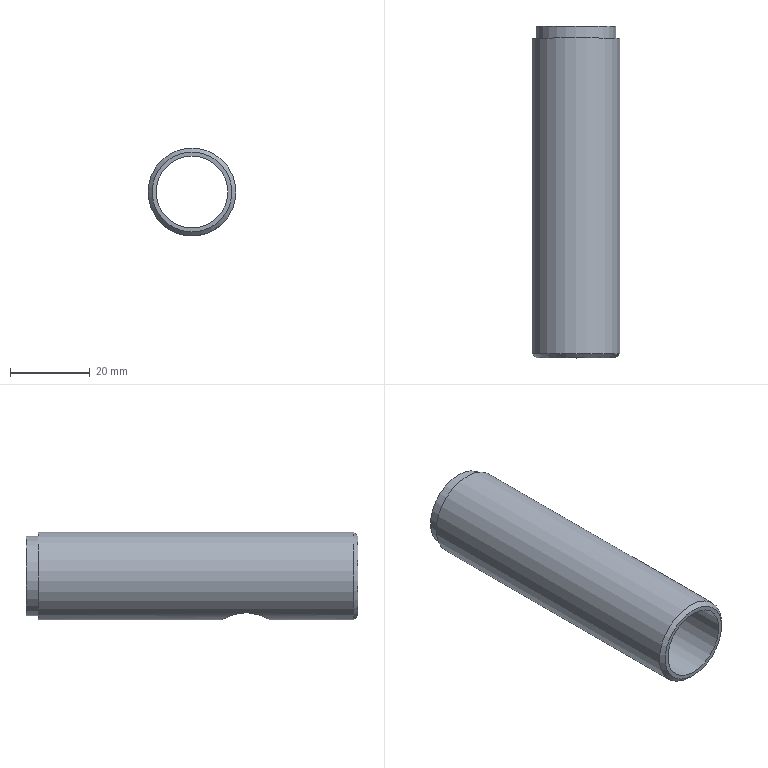Part | STEP file | JBJ-P-1012-04 | 1 solid | 8 faces | box 22 x 83 x 22 mm | volume 9931 mm3 | cylinder 4 | plane 2 | cone 2 | commonest cylinder face diameters 12 x1 18 x1 20 x1 22 x1
STEP:
#1=CARTESIAN_POINT('',(0.,0.,-10.));
#2=VERTEX_POINT('',#1);
#3=CARTESIAN_POINT('',(0.,0.,0.));
#4=DIRECTION('',(0.,-1.,0.));
#5=DIRECTION('',(0.,0.,-1.));
#6=AXIS2_PLACEMENT_3D('',#3,#4,#5);
#7=CIRCLE('',#6,10.);
#8=EDGE_CURVE('',#2,#2,#7,.T.);
#9=ORIENTED_EDGE('',*,*,#8,.T.);
#10=EDGE_LOOP('',(#9));
#11=FACE_OUTER_BOUND('',#10,.T.);
#12=CARTESIAN_POINT('',(0.,0.,-9.));
#13=VERTEX_POINT('',#12);
#14=CARTESIAN_POINT('',(0.,0.,0.));
#15=DIRECTION('',(0.,-1.,0.));
#16=DIRECTION('',(0.,0.,-1.));
#17=AXIS2_PLACEMENT_3D('',#14,#15,#16);
#18=CIRCLE('',#17,9.);
#19=EDGE_CURVE('',#13,#13,#18,.T.);
#20=ORIENTED_EDGE('',*,*,#19,.F.);
#21=EDGE_LOOP('',(#20));
#22=FACE_BOUND('',#21,.T.);
#23=CARTESIAN_POINT('',(11.,0.,0.));
#24=DIRECTION('',(0.,-1.,0.));
#25=DIRECTION('',(0.,0.,-1.));
#26=AXIS2_PLACEMENT_3D('',#23,#24,#25);
#27=PLANE('',#26);
#28=ADVANCED_FACE('',(#11,#22),#27,.T.);
#29=CARTESIAN_POINT('',(0.,34.,-9.));
#30=VERTEX_POINT('',#29);
#31=CARTESIAN_POINT('',(0.,34.,-9.));
#32=CARTESIAN_POINT('',(-0.4103,34.,-9.));
#33=CARTESIAN_POINT('',(-0.8115,33.958,-8.972));
#34=CARTESIAN_POINT('',(-1.597,33.797,-8.866));
#35=CARTESIAN_POINT('',(-1.985,33.676,-8.786));
#36=CARTESIAN_POINT('',(-2.708,33.368,-8.591));
#37=CARTESIAN_POINT('',(-3.05,33.182,-8.475));
#38=CARTESIAN_POINT('',(-3.692,32.746,-8.215));
#39=CARTESIAN_POINT('',(-3.984,32.502,-8.076));
#40=CARTESIAN_POINT('',(-4.519,31.965,-7.789));
#41=CARTESIAN_POINT('',(-4.763,31.668,-7.64));
#42=CARTESIAN_POINT('',(-5.188,31.039,-7.359));
#43=CARTESIAN_POINT('',(-5.37,30.705,-7.225));
#44=CARTESIAN_POINT('',(-5.673,29.992,-6.99));
#45=CARTESIAN_POINT('',(-5.794,29.609,-6.888));
#46=CARTESIAN_POINT('',(-5.916,29.023,-6.783));
#47=CARTESIAN_POINT('',(-5.947,28.825,-6.756));
#48=CARTESIAN_POINT('',(-5.989,28.421,-6.718));
#49=CARTESIAN_POINT('',(-6.,28.215,-6.709));
#50=CARTESIAN_POINT('',(-6.001,27.605,-6.708));
#51=CARTESIAN_POINT('',(-5.961,27.204,-6.744));
#52=CARTESIAN_POINT('',(-5.8,26.413,-6.882));
#53=CARTESIAN_POINT('',(-5.682,26.035,-6.982));
#54=CARTESIAN_POINT('',(-5.38,25.316,-7.217));
#55=CARTESIAN_POINT('',(-5.195,24.974,-7.354));
#56=CARTESIAN_POINT('',(-4.771,24.342,-7.636));
#57=CARTESIAN_POINT('',(-4.529,24.046,-7.783));
#58=CARTESIAN_POINT('',(-3.992,23.504,-8.072));
#59=CARTESIAN_POINT('',(-3.7,23.261,-8.211));
#60=CARTESIAN_POINT('',(-3.226,22.937,-8.404));
#61=CARTESIAN_POINT('',(-3.061,22.836,-8.465));
#62=CARTESIAN_POINT('',(-2.719,22.648,-8.581));
#63=CARTESIAN_POINT('',(-2.54,22.561,-8.636));
#64=CARTESIAN_POINT('',(-1.996,22.328,-8.784));
#65=CARTESIAN_POINT('',(-1.617,22.208,-8.863));
#66=CARTESIAN_POINT('',(-1.023,22.084,-8.944));
#67=CARTESIAN_POINT('',(-0.8202,22.053,-8.965));
#68=CARTESIAN_POINT('',(-0.4168,22.011,-8.993));
#69=CARTESIAN_POINT('',(-0.01304,21.99,-9.007));
#70=CARTESIAN_POINT('',(0.3916,22.009,-8.994));
#71=CARTESIAN_POINT('',(0.7967,22.05,-8.967));
#72=CARTESIAN_POINT('',(0.9997,22.08,-8.947));
#73=CARTESIAN_POINT('',(1.593,22.201,-8.867));
#74=CARTESIAN_POINT('',(1.973,22.32,-8.789));
#75=CARTESIAN_POINT('',(2.705,22.63,-8.592));
#76=CARTESIAN_POINT('',(3.048,22.818,-8.475));
#77=CARTESIAN_POINT('',(3.686,23.25,-8.218));
#78=CARTESIAN_POINT('',(3.985,23.498,-8.076));
#79=CARTESIAN_POINT('',(4.521,24.037,-7.788));
#80=CARTESIAN_POINT('',(4.761,24.329,-7.642));
#81=CARTESIAN_POINT('',(5.082,24.804,-7.429));
#82=CARTESIAN_POINT('',(5.182,24.969,-7.359));
#83=CARTESIAN_POINT('',(5.366,25.308,-7.227));
#84=CARTESIAN_POINT('',(5.449,25.482,-7.163));
#85=CARTESIAN_POINT('',(5.601,25.839,-7.046));
#86=CARTESIAN_POINT('',(5.668,26.022,-6.991));
#87=CARTESIAN_POINT('',(5.786,26.399,-6.894));
#88=CARTESIAN_POINT('',(5.837,26.595,-6.851));
#89=CARTESIAN_POINT('',(5.958,27.186,-6.746));
#90=CARTESIAN_POINT('',(6.,27.588,-6.708));
#91=CARTESIAN_POINT('',(6.,28.203,-6.708));
#92=CARTESIAN_POINT('',(5.99,28.408,-6.718));
#93=CARTESIAN_POINT('',(5.948,28.81,-6.754));
#94=CARTESIAN_POINT('',(5.918,29.009,-6.781));
#95=CARTESIAN_POINT('',(5.837,29.402,-6.85));
#96=CARTESIAN_POINT('',(5.787,29.597,-6.893));
#97=CARTESIAN_POINT('',(5.669,29.976,-6.991));
#98=CARTESIAN_POINT('',(5.601,30.16,-7.045));
#99=CARTESIAN_POINT('',(5.375,30.695,-7.222));
#100=CARTESIAN_POINT('',(5.192,31.032,-7.356));
#101=CARTESIAN_POINT('',(4.762,31.67,-7.641));
#102=CARTESIAN_POINT('',(4.522,31.962,-7.788));
#103=CARTESIAN_POINT('',(3.986,32.5,-8.075));
#104=CARTESIAN_POINT('',(3.688,32.748,-8.217));
#105=CARTESIAN_POINT('',(3.051,33.181,-8.474));
#106=CARTESIAN_POINT('',(2.713,33.366,-8.59));
#107=CARTESIAN_POINT('',(1.991,33.674,-8.785));
#108=CARTESIAN_POINT('',(1.602,33.796,-8.865));
#109=CARTESIAN_POINT('',(0.814,33.958,-8.972));
#110=CARTESIAN_POINT('',(0.4103,34.,-9.));
#111=CARTESIAN_POINT('',(0.,34.,-9.));
#112=B_SPLINE_CURVE_WITH_KNOTS('',3,(#31,#32,#33,#34,#35,#36,#37,#38,#39,#40,#41,#42,#43,#44,#45,#46,#47,#48,#49,#50,#51,#52,#53,#54,#55,#56,#57,#58,#59,#60,#61,#62,#63,#64,#65,#66,#67,#68,#69,#70,#71,#72,#73,#74,#75,#76,#77,#78,#79,#80,#81,#82,#83,#84,#85,#86,#87,#88,#89,#90,#91,#92,#93,#94,#95,#96,#97,#98,#99,#100,#101,#102,#103,#104,#105,#106,#107,#108,#109,#110,#111),.UNSPECIFIED.,.T.,.F.,(4,2,2,2,2,2,2,2,2,2,2,2,2,2,2,2,2,2,2,1,2,2,2,2,2,2,2,2,2,2,2,2,2,2,2,2,2,2,2,2,4),(0.,0.001211,0.002422,0.003634,0.004845,0.006056,0.007267,0.008478,0.009084,0.00969,0.0109,0.01211,0.01332,0.01453,0.01575,0.01635,0.01696,0.01817,0.01877,0.01938,0.01998,0.02059,0.0218,0.02301,0.02422,0.02543,0.02604,0.02665,0.02725,0.02786,0.02907,0.02967,0.03028,0.03089,0.03149,0.0327,0.03391,0.03512,0.03634,0.03755,0.03876),.UNSPECIFIED.);
#113=EDGE_CURVE('',#30,#30,#112,.T.);
#114=ORIENTED_EDGE('',*,*,#113,.F.);
#115=EDGE_LOOP('',(#114));
#116=FACE_BOUND('',#115,.T.);
#117=CARTESIAN_POINT('',(0.,82.,9.));
#118=VERTEX_POINT('',#117);
#119=CARTESIAN_POINT('',(0.,82.,0.));
#120=DIRECTION('',(0.,1.,0.));
#121=DIRECTION('',(0.,0.,1.));
#122=AXIS2_PLACEMENT_3D('',#119,#120,#121);
#123=CIRCLE('',#122,9.);
#124=EDGE_CURVE('',#118,#118,#123,.T.);
#125=ORIENTED_EDGE('',*,*,#124,.T.);
#126=EDGE_LOOP('',(#125));
#127=FACE_OUTER_BOUND('',#126,.T.);
#128=ORIENTED_EDGE('',*,*,#19,.T.);
#129=EDGE_LOOP('',(#128));
#130=FACE_OUTER_BOUND('',#129,.T.);
#131=CARTESIAN_POINT('',(0.,0.,0.));
#132=DIRECTION('',(0.,-1.,0.));
#133=DIRECTION('',(0.,0.,-1.));
#134=AXIS2_PLACEMENT_3D('',#131,#132,#133);
#135=CYLINDRICAL_SURFACE('',#134,9.);
#136=ADVANCED_FACE('',(#116,#127,#130),#135,.F.);
#137=CARTESIAN_POINT('',(0.,83.,-10.));
#138=VERTEX_POINT('',#137);
#139=CARTESIAN_POINT('',(0.,83.,0.));
#140=DIRECTION('',(0.,-1.,0.));
#141=DIRECTION('',(0.,0.,-1.));
#142=AXIS2_PLACEMENT_3D('',#139,#140,#141);
#143=CIRCLE('',#142,10.);
#144=EDGE_CURVE('',#138,#138,#143,.T.);
#145=ORIENTED_EDGE('',*,*,#144,.T.);
#146=EDGE_LOOP('',(#145));
#147=FACE_OUTER_BOUND('',#146,.T.);
#148=CARTESIAN_POINT('',(0.,80.,-10.));
#149=VERTEX_POINT('',#148);
#150=CARTESIAN_POINT('',(0.,80.,0.));
#151=DIRECTION('',(0.,-1.,0.));
#152=DIRECTION('',(0.,0.,-1.));
#153=AXIS2_PLACEMENT_3D('',#150,#151,#152);
#154=CIRCLE('',#153,10.);
#155=EDGE_CURVE('',#149,#149,#154,.T.);
#156=ORIENTED_EDGE('',*,*,#155,.F.);
#157=EDGE_LOOP('',(#156));
#158=FACE_OUTER_BOUND('',#157,.T.);
#159=CARTESIAN_POINT('',(0.,0.,0.));
#160=DIRECTION('',(0.,-1.,0.));
#161=DIRECTION('',(0.,0.,-1.));
#162=AXIS2_PLACEMENT_3D('',#159,#160,#161);
#163=CYLINDRICAL_SURFACE('',#162,10.);
#164=ADVANCED_FACE('',(#147,#158),#163,.T.);
#165=ORIENTED_EDGE('',*,*,#155,.T.);
#166=EDGE_LOOP('',(#165));
#167=FACE_BOUND('',#166,.T.);
#168=CARTESIAN_POINT('',(0.,80.,-11.));
#169=VERTEX_POINT('',#168);
#170=CARTESIAN_POINT('',(0.,80.,0.));
#171=DIRECTION('',(0.,-1.,0.));
#172=DIRECTION('',(0.,0.,-1.));
#173=AXIS2_PLACEMENT_3D('',#170,#171,#172);
#174=CIRCLE('',#173,11.);
#175=EDGE_CURVE('',#169,#169,#174,.T.);
#176=ORIENTED_EDGE('',*,*,#175,.F.);
#177=EDGE_LOOP('',(#176));
#178=FACE_OUTER_BOUND('',#177,.T.);
#179=CARTESIAN_POINT('',(10.,80.,0.));
#180=DIRECTION('',(0.,1.,0.));
#181=DIRECTION('',(0.,0.,1.));
#182=AXIS2_PLACEMENT_3D('',#179,#180,#181);
#183=PLANE('',#182);
#184=ADVANCED_FACE('',(#167,#178),#183,.T.);
#185=CARTESIAN_POINT('',(0.,34.,-11.));
#186=VERTEX_POINT('',#185);
#187=CARTESIAN_POINT('',(0.,34.,-11.));
#188=CARTESIAN_POINT('',(0.4049,34.,-11.));
#189=CARTESIAN_POINT('',(0.8015,33.959,-10.978));
#190=CARTESIAN_POINT('',(1.58,33.802,-10.893));
#191=CARTESIAN_POINT('',(1.965,33.683,-10.829));
#192=CARTESIAN_POINT('',(2.688,33.378,-10.673));
#193=CARTESIAN_POINT('',(3.03,33.193,-10.58));
#194=CARTESIAN_POINT('',(3.676,32.758,-10.373));
#195=CARTESIAN_POINT('',(3.974,32.511,-10.261));
#196=CARTESIAN_POINT('',(4.38,32.105,-10.091));
#197=CARTESIAN_POINT('',(4.509,31.963,-10.034));
#198=CARTESIAN_POINT('',(4.754,31.665,-9.921));
#199=CARTESIAN_POINT('',(4.87,31.509,-9.864));
#200=CARTESIAN_POINT('',(5.194,31.029,-9.7));
#201=CARTESIAN_POINT('',(5.377,30.69,-9.598));
#202=CARTESIAN_POINT('',(5.604,30.153,-9.466));
#203=CARTESIAN_POINT('',(5.671,29.969,-9.426));
#204=CARTESIAN_POINT('',(5.789,29.59,-9.354));
#205=CARTESIAN_POINT('',(5.839,29.396,-9.323));
#206=CARTESIAN_POINT('',(5.958,28.814,-9.247));
#207=CARTESIAN_POINT('',(5.999,28.42,-9.22));
#208=CARTESIAN_POINT('',(6.001,27.819,-9.219));
#209=CARTESIAN_POINT('',(5.991,27.615,-9.225));
#210=CARTESIAN_POINT('',(5.952,27.216,-9.251));
#211=CARTESIAN_POINT('',(5.922,27.018,-9.27));
#212=CARTESIAN_POINT('',(5.845,26.63,-9.319));
#213=CARTESIAN_POINT('',(5.796,26.438,-9.349));
#214=CARTESIAN_POINT('',(5.681,26.059,-9.42));
#215=CARTESIAN_POINT('',(5.613,25.872,-9.46));
#216=CARTESIAN_POINT('',(5.387,25.328,-9.592));
#217=CARTESIAN_POINT('',(5.203,24.987,-9.695));
#218=CARTESIAN_POINT('',(4.88,24.504,-9.859));
#219=CARTESIAN_POINT('',(4.764,24.348,-9.916));
#220=CARTESIAN_POINT('',(4.52,24.05,-10.029));
#221=CARTESIAN_POINT('',(4.392,23.907,-10.086));
#222=CARTESIAN_POINT('',(3.987,23.5,-10.256));
#223=CARTESIAN_POINT('',(3.69,23.252,-10.368));
#224=CARTESIAN_POINT('',(3.044,22.815,-10.576));
#225=CARTESIAN_POINT('',(2.703,22.629,-10.669));
#226=CARTESIAN_POINT('',(2.164,22.4,-10.787));
#227=CARTESIAN_POINT('',(1.98,22.333,-10.822));
#228=CARTESIAN_POINT('',(1.601,22.214,-10.885));
#229=CARTESIAN_POINT('',(1.406,22.164,-10.912));
#230=CARTESIAN_POINT('',(0.8187,22.043,-10.977));
#231=CARTESIAN_POINT('',(0.423,22.002,-10.999));
#232=CARTESIAN_POINT('',(-0.3772,21.999,-11.001));
#233=CARTESIAN_POINT('',(-0.784,22.038,-10.979));
#234=CARTESIAN_POINT('',(-1.564,22.194,-10.895));
#235=CARTESIAN_POINT('',(-1.946,22.31,-10.833));
#236=CARTESIAN_POINT('',(-2.677,22.616,-10.676));
#237=CARTESIAN_POINT('',(-3.02,22.801,-10.583));
#238=CARTESIAN_POINT('',(-3.664,23.233,-10.377));
#239=CARTESIAN_POINT('',(-3.966,23.482,-10.264));
#240=CARTESIAN_POINT('',(-4.51,24.024,-10.037));
#241=CARTESIAN_POINT('',(-4.754,24.319,-9.922));
#242=CARTESIAN_POINT('',(-5.189,24.963,-9.702));
#243=CARTESIAN_POINT('',(-5.375,25.305,-9.599));
#244=CARTESIAN_POINT('',(-5.677,26.021,-9.423));
#245=CARTESIAN_POINT('',(-5.796,26.397,-9.35));
#246=CARTESIAN_POINT('',(-5.958,27.184,-9.247));
#247=CARTESIAN_POINT('',(-5.999,27.58,-9.22));
#248=CARTESIAN_POINT('',(-6.001,28.178,-9.219));
#249=CARTESIAN_POINT('',(-5.991,28.378,-9.225));
#250=CARTESIAN_POINT('',(-5.953,28.78,-9.25));
#251=CARTESIAN_POINT('',(-5.923,28.98,-9.269));
#252=CARTESIAN_POINT('',(-5.806,29.566,-9.344));
#253=CARTESIAN_POINT('',(-5.69,29.943,-9.415));
#254=CARTESIAN_POINT('',(-5.386,30.673,-9.593));
#255=CARTESIAN_POINT('',(-5.202,31.016,-9.695));
#256=CARTESIAN_POINT('',(-4.772,31.658,-9.914));
#257=CARTESIAN_POINT('',(-4.524,31.96,-10.031));
#258=CARTESIAN_POINT('',(-3.982,32.505,-10.258));
#259=CARTESIAN_POINT('',(-3.686,32.75,-10.37));
#260=CARTESIAN_POINT('',(-3.203,33.077,-10.525));
#261=CARTESIAN_POINT('',(-3.034,33.18,-10.575));
#262=CARTESIAN_POINT('',(-2.69,33.367,-10.667));
#263=CARTESIAN_POINT('',(-2.514,33.451,-10.71));
#264=CARTESIAN_POINT('',(-1.974,33.68,-10.828));
#265=CARTESIAN_POINT('',(-1.598,33.797,-10.891));
#266=CARTESIAN_POINT('',(-0.8093,33.959,-10.977));
#267=CARTESIAN_POINT('',(-0.4049,34.,-11.));
#268=CARTESIAN_POINT('',(0.,34.,-11.));
#269=B_SPLINE_CURVE_WITH_KNOTS('',3,(#187,#188,#189,#190,#191,#192,#193,#194,#195,#196,#197,#198,#199,#200,#201,#202,#203,#204,#205,#206,#207,#208,#209,#210,#211,#212,#213,#214,#215,#216,#217,#218,#219,#220,#221,#222,#223,#224,#225,#226,#227,#228,#229,#230,#231,#232,#233,#234,#235,#236,#237,#238,#239,#240,#241,#242,#243,#244,#245,#246,#247,#248,#249,#250,#251,#252,#253,#254,#255,#256,#257,#258,#259,#260,#261,#262,#263,#264,#265,#266,#267,#268),.UNSPECIFIED.,.T.,.F.,(4,2,2,2,2,2,2,2,2,2,2,2,2,2,2,2,2,2,2,2,2,2,2,2,2,2,2,2,2,2,2,2,2,2,2,2,2,2,2,2,4),(0.,0.001196,0.002392,0.003588,0.004784,0.005382,0.00598,0.007175,0.007773,0.008371,0.009567,0.01017,0.01076,0.01136,0.01196,0.01315,0.01375,0.01435,0.01555,0.01674,0.01734,0.01794,0.01913,0.02033,0.02153,0.02272,0.02392,0.02511,0.02631,0.02751,0.0287,0.0293,0.0299,0.03109,0.03229,0.03349,0.03468,0.03528,0.03588,0.03707,0.03827),.UNSPECIFIED.);
#270=EDGE_CURVE('',#186,#186,#269,.T.);
#271=ORIENTED_EDGE('',*,*,#270,.F.);
#272=EDGE_LOOP('',(#271));
#273=FACE_BOUND('',#272,.T.);
#274=CARTESIAN_POINT('',(0.,1.,-11.));
#275=VERTEX_POINT('',#274);
#276=CARTESIAN_POINT('',(0.,1.,0.));
#277=DIRECTION('',(0.,1.,0.));
#278=DIRECTION('',(0.,0.,-1.));
#279=AXIS2_PLACEMENT_3D('',#276,#277,#278);
#280=CIRCLE('',#279,11.);
#281=EDGE_CURVE('',#275,#275,#280,.T.);
#282=ORIENTED_EDGE('',*,*,#281,.T.);
#283=EDGE_LOOP('',(#282));
#284=FACE_OUTER_BOUND('',#283,.T.);
#285=ORIENTED_EDGE('',*,*,#175,.T.);
#286=EDGE_LOOP('',(#285));
#287=FACE_OUTER_BOUND('',#286,.T.);
#288=CARTESIAN_POINT('',(0.,0.,0.));
#289=DIRECTION('',(0.,-1.,0.));
#290=DIRECTION('',(0.,0.,-1.));
#291=AXIS2_PLACEMENT_3D('',#288,#289,#290);
#292=CYLINDRICAL_SURFACE('',#291,11.);
#293=ADVANCED_FACE('',(#273,#284,#287),#292,.T.);
#294=ORIENTED_EDGE('',*,*,#281,.F.);
#295=EDGE_LOOP('',(#294));
#296=FACE_OUTER_BOUND('',#295,.T.);
#297=ORIENTED_EDGE('',*,*,#8,.F.);
#298=EDGE_LOOP('',(#297));
#299=FACE_BOUND('',#298,.T.);
#300=CARTESIAN_POINT('',(0.,0.,0.));
#301=DIRECTION('',(0.,1.,0.));
#302=DIRECTION('',(0.,0.,1.));
#303=AXIS2_PLACEMENT_3D('',#300,#301,#302);
#304=CONICAL_SURFACE('',#303,10.,0.7854);
#305=ADVANCED_FACE('',(#296,#299),#304,.T.);
#306=ORIENTED_EDGE('',*,*,#124,.F.);
#307=EDGE_LOOP('',(#306));
#308=FACE_BOUND('',#307,.T.);
#309=ORIENTED_EDGE('',*,*,#144,.F.);
#310=EDGE_LOOP('',(#309));
#311=FACE_OUTER_BOUND('',#310,.T.);
#312=CARTESIAN_POINT('',(0.,83.,0.));
#313=DIRECTION('',(0.,1.,0.));
#314=DIRECTION('',(0.,0.,1.));
#315=AXIS2_PLACEMENT_3D('',#312,#313,#314);
#316=CONICAL_SURFACE('',#315,10.,0.7854);
#317=ADVANCED_FACE('',(#308,#311),#316,.F.);
#318=ORIENTED_EDGE('',*,*,#113,.T.);
#319=EDGE_LOOP('',(#318));
#320=FACE_OUTER_BOUND('',#319,.T.);
#321=ORIENTED_EDGE('',*,*,#270,.T.);
#322=EDGE_LOOP('',(#321));
#323=FACE_OUTER_BOUND('',#322,.T.);
#324=CARTESIAN_POINT('',(0.,28.,-11.));
#325=DIRECTION('',(0.,0.,1.));
#326=DIRECTION('',(1.,0.,0.));
#327=AXIS2_PLACEMENT_3D('',#324,#325,#326);
#328=CYLINDRICAL_SURFACE('',#327,6.);
#329=ADVANCED_FACE('',(#320,#323),#328,.F.);
#330=CLOSED_SHELL('',(#28,#136,#164,#184,#293,#305,#317,#329));
#331=MANIFOLD_SOLID_BREP('',#330);
#332=CARTESIAN_POINT('',(0.,0.,0.));
#333=DIRECTION('',(0.,0.,1.));
#334=DIRECTION('',(1.,0.,0.));
#335=AXIS2_PLACEMENT_3D('',#332,#333,#334);
#336=(LENGTH_UNIT()NAMED_UNIT(*)SI_UNIT(.MILLI.,.METRE.));
#337=UNCERTAINTY_MEASURE_WITH_UNIT(LENGTH_MEASURE(0.00001),#336,'','');
#338=(NAMED_UNIT(*)PLANE_ANGLE_UNIT()SI_UNIT($,.RADIAN.));
#339=(NAMED_UNIT(*)SI_UNIT($,.STERADIAN.)SOLID_ANGLE_UNIT());
#340=(GEOMETRIC_REPRESENTATION_CONTEXT(3)GLOBAL_UNCERTAINTY_ASSIGNED_CONTEXT((#337))GLOBAL_UNIT_ASSIGNED_CONTEXT((#336,#338,#339))REPRESENTATION_CONTEXT('',''));
#341=ADVANCED_BREP_SHAPE_REPRESENTATION('',(#331,#335),#340);